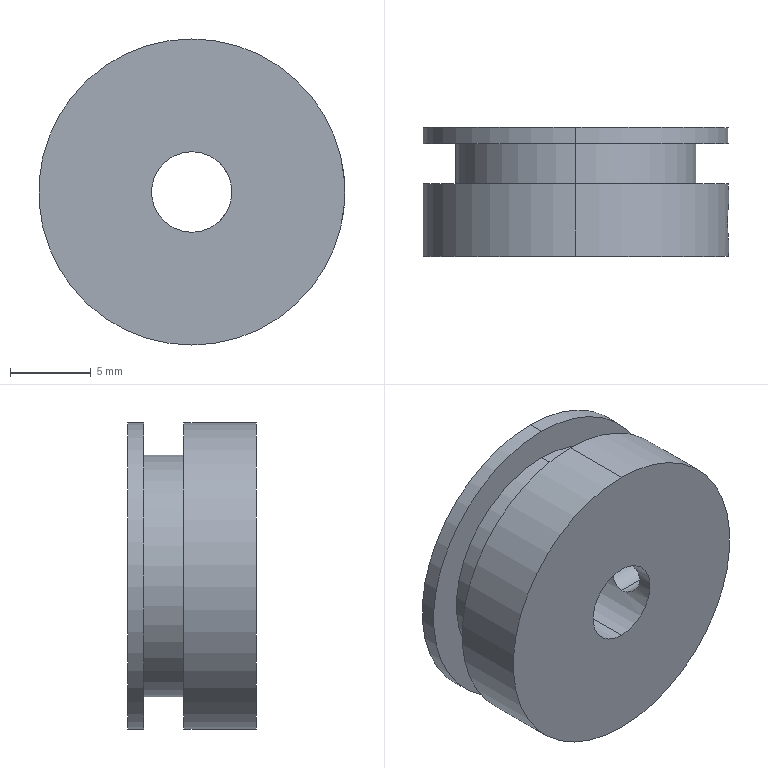Part | SolidWorks | features 3DProfileFeature 1, HoleWzd 1, Revolution 1 | 1 solid | 14 faces | box 19 x 8 x 19 mm | volume 1809 mm3 | cylinder 10 | plane 4 | commonest cylinder face diameters 19 x4 2.5 x2 5 x2 15 x2
STEP:
#1=CARTESIAN_POINT('',(2.168,-1.857,1.245));
#2=VERTEX_POINT('',#1);
#3=CARTESIAN_POINT('',(2.162,-1.857,-1.255));
#4=VERTEX_POINT('',#3);
#5=CARTESIAN_POINT('',(2.168,-1.857,1.245));
#6=CARTESIAN_POINT('',(2.168,-1.94,1.245));
#7=CARTESIAN_POINT('',(2.173,-2.024,1.237));
#8=CARTESIAN_POINT('',(2.191,-2.186,1.204));
#9=CARTESIAN_POINT('',(2.204,-2.265,1.18));
#10=CARTESIAN_POINT('',(2.254,-2.492,1.084));
#11=CARTESIAN_POINT('',(2.298,-2.628,0.9925));
#12=CARTESIAN_POINT('',(2.383,-2.855,0.7653));
#13=CARTESIAN_POINT('',(2.425,-2.947,0.6282));
#14=CARTESIAN_POINT('',(2.483,-3.073,0.3281));
#15=CARTESIAN_POINT('',(2.5,-3.107,0.1611));
#16=CARTESIAN_POINT('',(2.5,-3.107,-0.1698));
#17=CARTESIAN_POINT('',(2.482,-3.074,-0.3365));
#18=CARTESIAN_POINT('',(2.422,-2.947,-0.6395));
#19=CARTESIAN_POINT('',(2.38,-2.855,-0.7756));
#20=CARTESIAN_POINT('',(2.315,-2.683,-0.9466));
#21=CARTESIAN_POINT('',(2.293,-2.622,-0.9974));
#22=CARTESIAN_POINT('',(2.252,-2.488,-1.087));
#23=CARTESIAN_POINT('',(2.232,-2.415,-1.126));
#24=CARTESIAN_POINT('',(2.199,-2.265,-1.189));
#25=CARTESIAN_POINT('',(2.186,-2.188,-1.213));
#26=CARTESIAN_POINT('',(2.167,-2.026,-1.246));
#27=CARTESIAN_POINT('',(2.162,-1.941,-1.255));
#28=CARTESIAN_POINT('',(2.162,-1.857,-1.255));
#29=B_SPLINE_CURVE_WITH_KNOTS('',3,(#5,#6,#7,#8,#9,#10,#11,#12,#13,#14,#15,#16,#17,#18,#19,#20,#21,#22,#23,#24,#25,#26,#27,#28),.UNSPECIFIED.,.F.,.F.,(4,2,2,2,2,2,2,2,2,2,2,4),(0.003976,0.004224,0.004472,0.004968,0.005464,0.00596,0.006456,0.006952,0.0072,0.007448,0.007696,0.007944),.UNSPECIFIED.);
#30=EDGE_CURVE('',#2,#4,#29,.T.);
#31=ORIENTED_EDGE('',*,*,#30,.F.);
#32=CARTESIAN_POINT('',(9.42,-1.857,1.23));
#33=VERTEX_POINT('',#32);
#34=CARTESIAN_POINT('',(9.503,-1.857,1.229));
#35=DIRECTION('',(1.,0.,-0.002172));
#36=VECTOR('',#35,1000.);
#37=LINE('',#34,#36);
#38=EDGE_CURVE('',#2,#33,#37,.T.);
#39=ORIENTED_EDGE('',*,*,#38,.T.);
#40=CARTESIAN_POINT('',(9.415,-1.857,-1.27));
#41=VERTEX_POINT('',#40);
#42=CARTESIAN_POINT('',(9.415,-1.857,-1.27));
#43=CARTESIAN_POINT('',(9.415,-2.023,-1.27));
#44=CARTESIAN_POINT('',(9.419,-2.185,-1.238));
#45=CARTESIAN_POINT('',(9.435,-2.488,-1.112));
#46=CARTESIAN_POINT('',(9.446,-2.626,-1.019));
#47=CARTESIAN_POINT('',(9.468,-2.857,-0.7891));
#48=CARTESIAN_POINT('',(9.479,-2.95,-0.6497));
#49=CARTESIAN_POINT('',(9.495,-3.074,-0.349));
#50=CARTESIAN_POINT('',(9.5,-3.107,-0.1844));
#51=CARTESIAN_POINT('',(9.5,-3.107,0.06053));
#52=CARTESIAN_POINT('',(9.499,-3.099,0.1435));
#53=CARTESIAN_POINT('',(9.495,-3.067,0.3039));
#54=CARTESIAN_POINT('',(9.493,-3.044,0.3818));
#55=CARTESIAN_POINT('',(9.482,-2.949,0.609));
#56=CARTESIAN_POINT('',(9.471,-2.858,0.7466));
#57=CARTESIAN_POINT('',(9.45,-2.625,0.9799));
#58=CARTESIAN_POINT('',(9.44,-2.487,1.072));
#59=CARTESIAN_POINT('',(9.428,-2.26,1.166));
#60=CARTESIAN_POINT('',(9.425,-2.182,1.189));
#61=CARTESIAN_POINT('',(9.421,-2.022,1.221));
#62=CARTESIAN_POINT('',(9.42,-1.939,1.23));
#63=CARTESIAN_POINT('',(9.42,-1.857,1.23));
#64=B_SPLINE_CURVE_WITH_KNOTS('',3,(#42,#43,#44,#45,#46,#47,#48,#49,#50,#51,#52,#53,#54,#55,#56,#57,#58,#59,#60,#61,#62,#63),.UNSPECIFIED.,.F.,.F.,(4,2,2,2,2,2,2,2,2,2,4),(0.,0.000489,0.0009781,0.001467,0.001956,0.002201,0.002445,0.002934,0.003423,0.003668,0.003912),.UNSPECIFIED.);
#65=EDGE_CURVE('',#41,#33,#64,.T.);
#66=ORIENTED_EDGE('',*,*,#65,.F.);
#67=CARTESIAN_POINT('',(9.497,-1.857,-1.271));
#68=DIRECTION('',(1.,0.,-0.002172));
#69=VECTOR('',#68,1000.);
#70=LINE('',#67,#69);
#71=EDGE_CURVE('',#4,#41,#70,.T.);
#72=ORIENTED_EDGE('',*,*,#71,.F.);
#73=EDGE_LOOP('',(#31,#39,#66,#72));
#74=FACE_OUTER_BOUND('',#73,.T.);
#75=CARTESIAN_POINT('',(9.5,-1.857,-0.02064));
#76=DIRECTION('',(1.,0.,-0.002172));
#77=DIRECTION('',(-0.002172,0.,-1.));
#78=AXIS2_PLACEMENT_3D('',#75,#76,#77);
#79=CYLINDRICAL_SURFACE('',#78,1.25);
#80=ADVANCED_FACE('',(#74),#79,.F.);
#81=CARTESIAN_POINT('',(0.,-4.,-2.5));
#82=VERTEX_POINT('',#81);
#83=CARTESIAN_POINT('',(0.,-4.,2.5));
#84=VERTEX_POINT('',#83);
#85=CARTESIAN_POINT('',(0.,-4.,0.));
#86=DIRECTION('',(0.,1.,0.));
#87=DIRECTION('',(0.,0.,1.));
#88=AXIS2_PLACEMENT_3D('',#85,#86,#87);
#89=CIRCLE('',#88,2.5);
#90=EDGE_CURVE('',#82,#84,#89,.T.);
#91=ORIENTED_EDGE('',*,*,#90,.F.);
#92=CARTESIAN_POINT('',(0.,4.,-2.5));
#93=VERTEX_POINT('',#92);
#94=CARTESIAN_POINT('',(0.,34.072,-2.5));
#95=DIRECTION('',(0.,1.,0.));
#96=VECTOR('',#95,1000.);
#97=LINE('',#94,#96);
#98=EDGE_CURVE('',#82,#93,#97,.T.);
#99=ORIENTED_EDGE('',*,*,#98,.T.);
#100=CARTESIAN_POINT('',(0.,4.,2.5));
#101=VERTEX_POINT('',#100);
#102=CARTESIAN_POINT('',(0.,4.,0.));
#103=DIRECTION('',(0.,1.,0.));
#104=DIRECTION('',(0.,0.,1.));
#105=AXIS2_PLACEMENT_3D('',#102,#103,#104);
#106=CIRCLE('',#105,2.5);
#107=EDGE_CURVE('',#93,#101,#106,.T.);
#108=ORIENTED_EDGE('',*,*,#107,.T.);
#109=CARTESIAN_POINT('',(0.,34.072,2.5));
#110=DIRECTION('',(0.,1.,0.));
#111=VECTOR('',#110,1000.);
#112=LINE('',#109,#111);
#113=EDGE_CURVE('',#84,#101,#112,.T.);
#114=ORIENTED_EDGE('',*,*,#113,.F.);
#115=EDGE_LOOP('',(#91,#99,#108,#114));
#116=FACE_OUTER_BOUND('',#115,.T.);
#117=CARTESIAN_POINT('',(0.,34.072,0.));
#118=DIRECTION('',(0.,1.,0.));
#119=DIRECTION('',(0.,0.,1.));
#120=AXIS2_PLACEMENT_3D('',#117,#118,#119);
#121=CYLINDRICAL_SURFACE('',#120,2.5);
#122=ADVANCED_FACE('',(#116),#121,.F.);
#123=ORIENTED_EDGE('',*,*,#65,.T.);
#124=CARTESIAN_POINT('',(9.42,-1.857,1.23));
#125=CARTESIAN_POINT('',(9.42,-1.694,1.23));
#126=CARTESIAN_POINT('',(9.425,-1.529,1.197));
#127=CARTESIAN_POINT('',(9.44,-1.229,1.072));
#128=CARTESIAN_POINT('',(9.45,-1.089,0.9791));
#129=CARTESIAN_POINT('',(9.466,-0.9163,0.8063));
#130=CARTESIAN_POINT('',(9.471,-0.8636,0.7421));
#131=CARTESIAN_POINT('',(9.481,-0.7729,0.6064));
#132=CARTESIAN_POINT('',(9.485,-0.7344,0.5347));
#133=CARTESIAN_POINT('',(9.496,-0.6401,0.3077));
#134=CARTESIAN_POINT('',(9.5,-0.6074,0.1455));
#135=CARTESIAN_POINT('',(9.5,-0.6072,-0.185));
#136=CARTESIAN_POINT('',(9.495,-0.6397,-0.3474));
#137=CARTESIAN_POINT('',(9.479,-0.765,-0.65));
#138=CARTESIAN_POINT('',(9.468,-0.8577,-0.7886));
#139=CARTESIAN_POINT('',(9.446,-1.088,-1.019));
#140=CARTESIAN_POINT('',(9.435,-1.227,-1.112));
#141=CARTESIAN_POINT('',(9.419,-1.528,-1.237));
#142=CARTESIAN_POINT('',(9.415,-1.692,-1.27));
#143=CARTESIAN_POINT('',(9.415,-1.857,-1.27));
#144=B_SPLINE_CURVE_WITH_KNOTS('',3,(#124,#125,#126,#127,#128,#129,#130,#131,#132,#133,#134,#135,#136,#137,#138,#139,#140,#141,#142,#143),.UNSPECIFIED.,.F.,.F.,(4,2,2,2,2,2,2,2,2,4),(0.003912,0.004401,0.00489,0.005135,0.005379,0.005868,0.006357,0.006846,0.007335,0.007824),.UNSPECIFIED.);
#145=EDGE_CURVE('',#33,#41,#144,.T.);
#146=ORIENTED_EDGE('',*,*,#145,.T.);
#147=EDGE_LOOP('',(#123,#146));
#148=FACE_BOUND('',#147,.T.);
#149=CARTESIAN_POINT('',(0.,-4.,9.5));
#150=VERTEX_POINT('',#149);
#151=CARTESIAN_POINT('',(0.,-4.,-9.5));
#152=VERTEX_POINT('',#151);
#153=CARTESIAN_POINT('',(0.,-4.,0.));
#154=DIRECTION('',(0.,1.,0.));
#155=DIRECTION('',(0.,0.,1.));
#156=AXIS2_PLACEMENT_3D('',#153,#154,#155);
#157=CIRCLE('',#156,9.5);
#158=EDGE_CURVE('',#150,#152,#157,.T.);
#159=ORIENTED_EDGE('',*,*,#158,.T.);
#160=CARTESIAN_POINT('',(0.,0.5,-9.5));
#161=VERTEX_POINT('',#160);
#162=CARTESIAN_POINT('',(0.,34.072,-9.5));
#163=DIRECTION('',(0.,1.,0.));
#164=VECTOR('',#163,1000.);
#165=LINE('',#162,#164);
#166=EDGE_CURVE('',#152,#161,#165,.T.);
#167=ORIENTED_EDGE('',*,*,#166,.T.);
#168=CARTESIAN_POINT('',(0.,0.5,9.5));
#169=VERTEX_POINT('',#168);
#170=CARTESIAN_POINT('',(0.,0.5,0.));
#171=DIRECTION('',(0.,1.,0.));
#172=DIRECTION('',(0.,0.,1.));
#173=AXIS2_PLACEMENT_3D('',#170,#171,#172);
#174=CIRCLE('',#173,9.5);
#175=EDGE_CURVE('',#169,#161,#174,.T.);
#176=ORIENTED_EDGE('',*,*,#175,.F.);
#177=CARTESIAN_POINT('',(0.,34.072,9.5));
#178=DIRECTION('',(0.,1.,0.));
#179=VECTOR('',#178,1000.);
#180=LINE('',#177,#179);
#181=EDGE_CURVE('',#150,#169,#180,.T.);
#182=ORIENTED_EDGE('',*,*,#181,.F.);
#183=EDGE_LOOP('',(#159,#167,#176,#182));
#184=FACE_OUTER_BOUND('',#183,.T.);
#185=CARTESIAN_POINT('',(0.,34.072,0.));
#186=DIRECTION('',(0.,1.,0.));
#187=DIRECTION('',(0.,0.,1.));
#188=AXIS2_PLACEMENT_3D('',#185,#186,#187);
#189=CYLINDRICAL_SURFACE('',#188,9.5);
#190=ADVANCED_FACE('',(#148,#184),#189,.T.);
#191=CARTESIAN_POINT('',(0.,0.5,7.5));
#192=VERTEX_POINT('',#191);
#193=CARTESIAN_POINT('',(0.,0.5,-7.5));
#194=VERTEX_POINT('',#193);
#195=CARTESIAN_POINT('',(0.,0.5,0.));
#196=DIRECTION('',(0.,1.,0.));
#197=DIRECTION('',(0.,0.,1.));
#198=AXIS2_PLACEMENT_3D('',#195,#196,#197);
#199=CIRCLE('',#198,7.5);
#200=EDGE_CURVE('',#192,#194,#199,.T.);
#201=ORIENTED_EDGE('',*,*,#200,.T.);
#202=CARTESIAN_POINT('',(0.,3.,-7.5));
#203=VERTEX_POINT('',#202);
#204=CARTESIAN_POINT('',(0.,34.072,-7.5));
#205=DIRECTION('',(0.,1.,0.));
#206=VECTOR('',#205,1000.);
#207=LINE('',#204,#206);
#208=EDGE_CURVE('',#194,#203,#207,.T.);
#209=ORIENTED_EDGE('',*,*,#208,.T.);
#210=CARTESIAN_POINT('',(0.,3.,7.5));
#211=VERTEX_POINT('',#210);
#212=CARTESIAN_POINT('',(0.,3.,0.));
#213=DIRECTION('',(0.,1.,0.));
#214=DIRECTION('',(0.,0.,1.));
#215=AXIS2_PLACEMENT_3D('',#212,#213,#214);
#216=CIRCLE('',#215,7.5);
#217=EDGE_CURVE('',#211,#203,#216,.T.);
#218=ORIENTED_EDGE('',*,*,#217,.F.);
#219=CARTESIAN_POINT('',(0.,34.072,7.5));
#220=DIRECTION('',(0.,1.,0.));
#221=VECTOR('',#220,1000.);
#222=LINE('',#219,#221);
#223=EDGE_CURVE('',#192,#211,#222,.T.);
#224=ORIENTED_EDGE('',*,*,#223,.F.);
#225=EDGE_LOOP('',(#201,#209,#218,#224));
#226=FACE_OUTER_BOUND('',#225,.T.);
#227=CARTESIAN_POINT('',(0.,34.072,0.));
#228=DIRECTION('',(0.,1.,0.));
#229=DIRECTION('',(0.,0.,1.));
#230=AXIS2_PLACEMENT_3D('',#227,#228,#229);
#231=CYLINDRICAL_SURFACE('',#230,7.5);
#232=ADVANCED_FACE('',(#226),#231,.T.);
#233=CARTESIAN_POINT('',(0.,3.,9.5));
#234=VERTEX_POINT('',#233);
#235=CARTESIAN_POINT('',(0.,3.,-9.5));
#236=VERTEX_POINT('',#235);
#237=CARTESIAN_POINT('',(0.,3.,0.));
#238=DIRECTION('',(0.,1.,0.));
#239=DIRECTION('',(0.,0.,1.));
#240=AXIS2_PLACEMENT_3D('',#237,#238,#239);
#241=CIRCLE('',#240,9.5);
#242=EDGE_CURVE('',#234,#236,#241,.T.);
#243=ORIENTED_EDGE('',*,*,#242,.T.);
#244=CARTESIAN_POINT('',(0.,4.,-9.5));
#245=VERTEX_POINT('',#244);
#246=CARTESIAN_POINT('',(0.,34.072,-9.5));
#247=DIRECTION('',(0.,1.,0.));
#248=VECTOR('',#247,1000.);
#249=LINE('',#246,#248);
#250=EDGE_CURVE('',#236,#245,#249,.T.);
#251=ORIENTED_EDGE('',*,*,#250,.T.);
#252=CARTESIAN_POINT('',(0.,4.,9.5));
#253=VERTEX_POINT('',#252);
#254=CARTESIAN_POINT('',(0.,4.,0.));
#255=DIRECTION('',(0.,1.,0.));
#256=DIRECTION('',(0.,0.,1.));
#257=AXIS2_PLACEMENT_3D('',#254,#255,#256);
#258=CIRCLE('',#257,9.5);
#259=EDGE_CURVE('',#253,#245,#258,.T.);
#260=ORIENTED_EDGE('',*,*,#259,.F.);
#261=CARTESIAN_POINT('',(0.,34.072,9.5));
#262=DIRECTION('',(0.,1.,0.));
#263=VECTOR('',#262,1000.);
#264=LINE('',#261,#263);
#265=EDGE_CURVE('',#234,#253,#264,.T.);
#266=ORIENTED_EDGE('',*,*,#265,.F.);
#267=EDGE_LOOP('',(#243,#251,#260,#266));
#268=FACE_OUTER_BOUND('',#267,.T.);
#269=CARTESIAN_POINT('',(0.,34.072,0.));
#270=DIRECTION('',(0.,1.,0.));
#271=DIRECTION('',(0.,0.,1.));
#272=AXIS2_PLACEMENT_3D('',#269,#270,#271);
#273=CYLINDRICAL_SURFACE('',#272,9.5);
#274=ADVANCED_FACE('',(#268),#273,.T.);
#275=CARTESIAN_POINT('',(0.,4.,0.));
#276=DIRECTION('',(0.,1.,0.));
#277=DIRECTION('',(0.,0.,1.));
#278=AXIS2_PLACEMENT_3D('',#275,#276,#277);
#279=CIRCLE('',#278,2.5);
#280=EDGE_CURVE('',#101,#93,#279,.T.);
#281=ORIENTED_EDGE('',*,*,#280,.F.);
#282=ORIENTED_EDGE('',*,*,#107,.F.);
#283=EDGE_LOOP('',(#281,#282));
#284=FACE_BOUND('',#283,.T.);
#285=ORIENTED_EDGE('',*,*,#259,.T.);
#286=CARTESIAN_POINT('',(0.,4.,0.));
#287=DIRECTION('',(0.,1.,0.));
#288=DIRECTION('',(0.,0.,1.));
#289=AXIS2_PLACEMENT_3D('',#286,#287,#288);
#290=CIRCLE('',#289,9.5);
#291=EDGE_CURVE('',#245,#253,#290,.T.);
#292=ORIENTED_EDGE('',*,*,#291,.T.);
#293=EDGE_LOOP('',(#285,#292));
#294=FACE_OUTER_BOUND('',#293,.T.);
#295=CARTESIAN_POINT('',(2.5,4.,0.));
#296=DIRECTION('',(0.,-1.,0.));
#297=DIRECTION('',(0.,0.,-1.));
#298=AXIS2_PLACEMENT_3D('',#295,#296,#297);
#299=PLANE('',#298);
#300=ADVANCED_FACE('',(#284,#294),#299,.F.);
#301=ORIENTED_EDGE('',*,*,#250,.F.);
#302=CARTESIAN_POINT('',(0.,3.,0.));
#303=DIRECTION('',(0.,1.,0.));
#304=DIRECTION('',(0.,0.,1.));
#305=AXIS2_PLACEMENT_3D('',#302,#303,#304);
#306=CIRCLE('',#305,9.5);
#307=EDGE_CURVE('',#236,#234,#306,.T.);
#308=ORIENTED_EDGE('',*,*,#307,.T.);
#309=ORIENTED_EDGE('',*,*,#265,.T.);
#310=ORIENTED_EDGE('',*,*,#291,.F.);
#311=EDGE_LOOP('',(#301,#308,#309,#310));
#312=FACE_OUTER_BOUND('',#311,.T.);
#313=CARTESIAN_POINT('',(0.,34.072,0.));
#314=DIRECTION('',(0.,1.,0.));
#315=DIRECTION('',(0.,0.,1.));
#316=AXIS2_PLACEMENT_3D('',#313,#314,#315);
#317=CYLINDRICAL_SURFACE('',#316,9.5);
#318=ADVANCED_FACE('',(#312),#317,.T.);
#319=ORIENTED_EDGE('',*,*,#242,.F.);
#320=ORIENTED_EDGE('',*,*,#307,.F.);
#321=EDGE_LOOP('',(#319,#320));
#322=FACE_OUTER_BOUND('',#321,.T.);
#323=ORIENTED_EDGE('',*,*,#217,.T.);
#324=CARTESIAN_POINT('',(0.,3.,0.));
#325=DIRECTION('',(0.,1.,0.));
#326=DIRECTION('',(0.,0.,1.));
#327=AXIS2_PLACEMENT_3D('',#324,#325,#326);
#328=CIRCLE('',#327,7.5);
#329=EDGE_CURVE('',#203,#211,#328,.T.);
#330=ORIENTED_EDGE('',*,*,#329,.T.);
#331=EDGE_LOOP('',(#323,#330));
#332=FACE_BOUND('',#331,.T.);
#333=CARTESIAN_POINT('',(9.5,3.,0.));
#334=DIRECTION('',(0.,1.,0.));
#335=DIRECTION('',(0.,0.,1.));
#336=AXIS2_PLACEMENT_3D('',#333,#334,#335);
#337=PLANE('',#336);
#338=ADVANCED_FACE('',(#322,#332),#337,.F.);
#339=ORIENTED_EDGE('',*,*,#208,.F.);
#340=CARTESIAN_POINT('',(0.,0.5,0.));
#341=DIRECTION('',(0.,1.,0.));
#342=DIRECTION('',(0.,0.,1.));
#343=AXIS2_PLACEMENT_3D('',#340,#341,#342);
#344=CIRCLE('',#343,7.5);
#345=EDGE_CURVE('',#194,#192,#344,.T.);
#346=ORIENTED_EDGE('',*,*,#345,.T.);
#347=ORIENTED_EDGE('',*,*,#223,.T.);
#348=ORIENTED_EDGE('',*,*,#329,.F.);
#349=EDGE_LOOP('',(#339,#346,#347,#348));
#350=FACE_OUTER_BOUND('',#349,.T.);
#351=CARTESIAN_POINT('',(0.,34.072,0.));
#352=DIRECTION('',(0.,1.,0.));
#353=DIRECTION('',(0.,0.,1.));
#354=AXIS2_PLACEMENT_3D('',#351,#352,#353);
#355=CYLINDRICAL_SURFACE('',#354,7.5);
#356=ADVANCED_FACE('',(#350),#355,.T.);
#357=ORIENTED_EDGE('',*,*,#200,.F.);
#358=ORIENTED_EDGE('',*,*,#345,.F.);
#359=EDGE_LOOP('',(#357,#358));
#360=FACE_BOUND('',#359,.T.);
#361=ORIENTED_EDGE('',*,*,#175,.T.);
#362=CARTESIAN_POINT('',(0.,0.5,0.));
#363=DIRECTION('',(0.,1.,0.));
#364=DIRECTION('',(0.,0.,1.));
#365=AXIS2_PLACEMENT_3D('',#362,#363,#364);
#366=CIRCLE('',#365,9.5);
#367=EDGE_CURVE('',#161,#169,#366,.T.);
#368=ORIENTED_EDGE('',*,*,#367,.T.);
#369=EDGE_LOOP('',(#361,#368));
#370=FACE_OUTER_BOUND('',#369,.T.);
#371=CARTESIAN_POINT('',(7.5,0.5,0.));
#372=DIRECTION('',(0.,-1.,0.));
#373=DIRECTION('',(0.,0.,-1.));
#374=AXIS2_PLACEMENT_3D('',#371,#372,#373);
#375=PLANE('',#374);
#376=ADVANCED_FACE('',(#360,#370),#375,.F.);
#377=ORIENTED_EDGE('',*,*,#166,.F.);
#378=CARTESIAN_POINT('',(0.,-4.,0.));
#379=DIRECTION('',(0.,1.,0.));
#380=DIRECTION('',(0.,0.,1.));
#381=AXIS2_PLACEMENT_3D('',#378,#379,#380);
#382=CIRCLE('',#381,9.5);
#383=EDGE_CURVE('',#152,#150,#382,.T.);
#384=ORIENTED_EDGE('',*,*,#383,.T.);
#385=ORIENTED_EDGE('',*,*,#181,.T.);
#386=ORIENTED_EDGE('',*,*,#367,.F.);
#387=EDGE_LOOP('',(#377,#384,#385,#386));
#388=FACE_OUTER_BOUND('',#387,.T.);
#389=CARTESIAN_POINT('',(0.,34.072,0.));
#390=DIRECTION('',(0.,1.,0.));
#391=DIRECTION('',(0.,0.,1.));
#392=AXIS2_PLACEMENT_3D('',#389,#390,#391);
#393=CYLINDRICAL_SURFACE('',#392,9.5);
#394=ADVANCED_FACE('',(#388),#393,.T.);
#395=ORIENTED_EDGE('',*,*,#158,.F.);
#396=ORIENTED_EDGE('',*,*,#383,.F.);
#397=EDGE_LOOP('',(#395,#396));
#398=FACE_OUTER_BOUND('',#397,.T.);
#399=CARTESIAN_POINT('',(0.,-4.,0.));
#400=DIRECTION('',(0.,1.,0.));
#401=DIRECTION('',(0.,0.,1.));
#402=AXIS2_PLACEMENT_3D('',#399,#400,#401);
#403=CIRCLE('',#402,2.5);
#404=EDGE_CURVE('',#84,#82,#403,.T.);
#405=ORIENTED_EDGE('',*,*,#404,.T.);
#406=ORIENTED_EDGE('',*,*,#90,.T.);
#407=EDGE_LOOP('',(#405,#406));
#408=FACE_BOUND('',#407,.T.);
#409=CARTESIAN_POINT('',(9.5,-4.,0.));
#410=DIRECTION('',(0.,1.,0.));
#411=DIRECTION('',(0.,0.,1.));
#412=AXIS2_PLACEMENT_3D('',#409,#410,#411);
#413=PLANE('',#412);
#414=ADVANCED_FACE('',(#398,#408),#413,.F.);
#415=ORIENTED_EDGE('',*,*,#98,.F.);
#416=ORIENTED_EDGE('',*,*,#404,.F.);
#417=ORIENTED_EDGE('',*,*,#113,.T.);
#418=ORIENTED_EDGE('',*,*,#280,.T.);
#419=EDGE_LOOP('',(#415,#416,#417,#418));
#420=FACE_OUTER_BOUND('',#419,.T.);
#421=CARTESIAN_POINT('',(2.162,-1.857,-1.255));
#422=CARTESIAN_POINT('',(2.162,-1.773,-1.255));
#423=CARTESIAN_POINT('',(2.167,-1.691,-1.246));
#424=CARTESIAN_POINT('',(2.186,-1.529,-1.214));
#425=CARTESIAN_POINT('',(2.199,-1.449,-1.189));
#426=CARTESIAN_POINT('',(2.249,-1.223,-1.095));
#427=CARTESIAN_POINT('',(2.293,-1.087,-1.003));
#428=CARTESIAN_POINT('',(2.38,-0.8604,-0.7761));
#429=CARTESIAN_POINT('',(2.422,-0.7678,-0.6393));
#430=CARTESIAN_POINT('',(2.467,-0.6732,-0.4141));
#431=CARTESIAN_POINT('',(2.479,-0.6484,-0.3339));
#432=CARTESIAN_POINT('',(2.495,-0.6156,-0.1717));
#433=CARTESIAN_POINT('',(2.5,-0.6073,-0.08955));
#434=CARTESIAN_POINT('',(2.5,-0.6072,0.1604));
#435=CARTESIAN_POINT('',(2.483,-0.641,0.3268));
#436=CARTESIAN_POINT('',(2.424,-0.7685,0.6306));
#437=CARTESIAN_POINT('',(2.383,-0.8612,0.7669));
#438=CARTESIAN_POINT('',(2.297,-1.089,0.9936));
#439=CARTESIAN_POINT('',(2.253,-1.225,1.086));
#440=CARTESIAN_POINT('',(2.188,-1.525,1.211));
#441=CARTESIAN_POINT('',(2.168,-1.691,1.245));
#442=CARTESIAN_POINT('',(2.168,-1.857,1.245));
#443=B_SPLINE_CURVE_WITH_KNOTS('',3,(#421,#422,#423,#424,#425,#426,#427,#428,#429,#430,#431,#432,#433,#434,#435,#436,#437,#438,#439,#440,#441,#442),.UNSPECIFIED.,.F.,.F.,(4,2,2,2,2,2,2,2,2,2,4),(0.,0.0002485,0.000497,0.0009939,0.001491,0.001739,0.001988,0.002485,0.002982,0.003479,0.003976),.UNSPECIFIED.);
#444=EDGE_CURVE('',#4,#2,#443,.T.);
#445=ORIENTED_EDGE('',*,*,#444,.T.);
#446=ORIENTED_EDGE('',*,*,#30,.T.);
#447=EDGE_LOOP('',(#445,#446));
#448=FACE_BOUND('',#447,.T.);
#449=CARTESIAN_POINT('',(0.,34.072,0.));
#450=DIRECTION('',(0.,1.,0.));
#451=DIRECTION('',(0.,0.,1.));
#452=AXIS2_PLACEMENT_3D('',#449,#450,#451);
#453=CYLINDRICAL_SURFACE('',#452,2.5);
#454=ADVANCED_FACE('',(#420,#448),#453,.F.);
#455=ORIENTED_EDGE('',*,*,#38,.F.);
#456=ORIENTED_EDGE('',*,*,#444,.F.);
#457=ORIENTED_EDGE('',*,*,#71,.T.);
#458=ORIENTED_EDGE('',*,*,#145,.F.);
#459=EDGE_LOOP('',(#455,#456,#457,#458));
#460=FACE_OUTER_BOUND('',#459,.T.);
#461=CARTESIAN_POINT('',(9.5,-1.857,-0.02064));
#462=DIRECTION('',(1.,0.,-0.002172));
#463=DIRECTION('',(-0.002172,0.,-1.));
#464=AXIS2_PLACEMENT_3D('',#461,#462,#463);
#465=CYLINDRICAL_SURFACE('',#464,1.25);
#466=ADVANCED_FACE('',(#460),#465,.F.);
#467=CLOSED_SHELL('',(#80,#122,#190,#232,#274,#300,#318,#338,#356,#376,#394,#414,#454,#466));
#468=MANIFOLD_SOLID_BREP('',#467);
#469=CARTESIAN_POINT('',(0.,0.,0.));
#470=DIRECTION('',(0.,0.,1.));
#471=DIRECTION('',(1.,0.,0.));
#472=AXIS2_PLACEMENT_3D('',#469,#470,#471);
#473=(LENGTH_UNIT()NAMED_UNIT(*)SI_UNIT(.MILLI.,.METRE.));
#474=UNCERTAINTY_MEASURE_WITH_UNIT(LENGTH_MEASURE(0.00001),#473,'','');
#475=(NAMED_UNIT(*)PLANE_ANGLE_UNIT()SI_UNIT($,.RADIAN.));
#476=(NAMED_UNIT(*)SI_UNIT($,.STERADIAN.)SOLID_ANGLE_UNIT());
#477=(GEOMETRIC_REPRESENTATION_CONTEXT(3)GLOBAL_UNCERTAINTY_ASSIGNED_CONTEXT((#474))GLOBAL_UNIT_ASSIGNED_CONTEXT((#473,#475,#476))REPRESENTATION_CONTEXT('',''));
#478=ADVANCED_BREP_SHAPE_REPRESENTATION('',(#468,#472),#477);